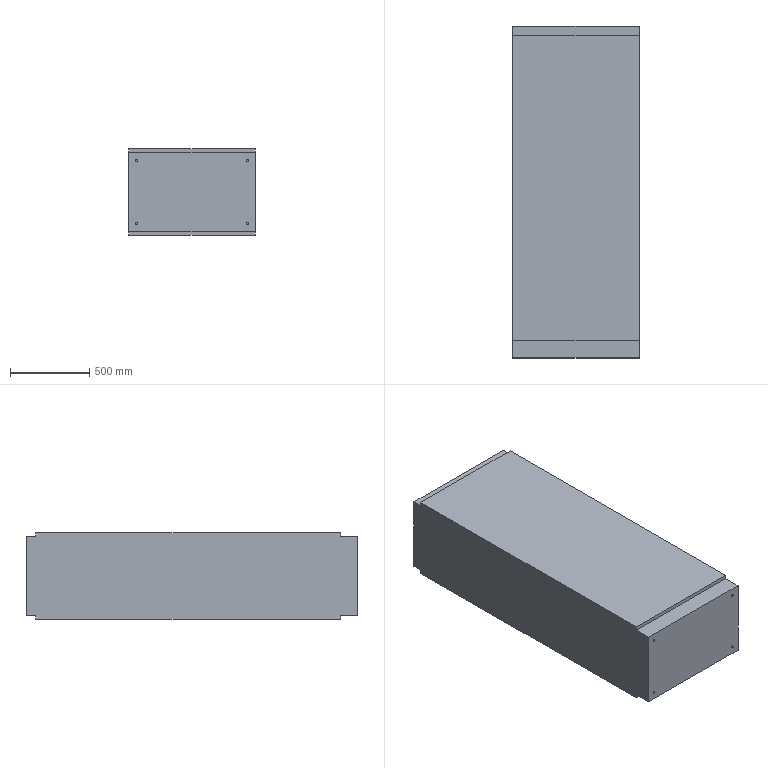Part | STEP file | Power distribution cabinet | 1 solid | 255 faces | box 800 x 2100 x 550 mm | volume 917054924 mm3 | plane 154 | spline 93 | cylinder 8 | commonest cylinder face diameters 14 x8